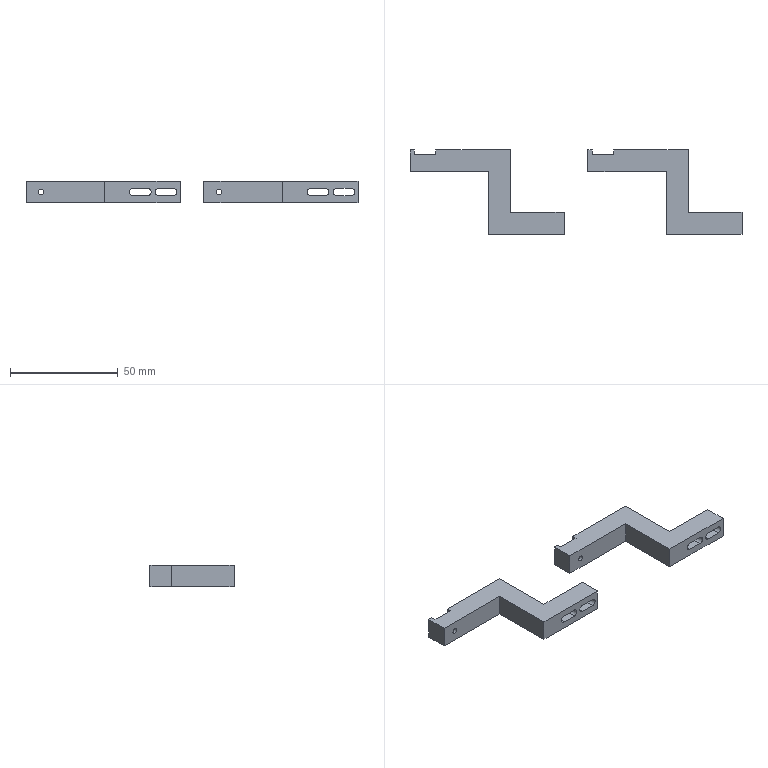Part | 2 solids | 46 faces | box 154 x 39 x 10 mm | volume 18361 mm3 | plane 36 | cylinder 10 | commonest cylinder face diameters 3.4 x8 2.5 x2
STEP:
#1=CARTESIAN_POINT('',(-3.2,10.,6.7));
#2=VERTEX_POINT('',#1);
#3=CARTESIAN_POINT('',(-3.2,0.,6.7));
#4=VERTEX_POINT('',#3);
#5=CARTESIAN_POINT('',(-3.2,10.,6.7));
#6=DIRECTION('',(0.,-1.,0.));
#7=VECTOR('',#6,1000.);
#8=LINE('',#5,#7);
#9=EDGE_CURVE('',#2,#4,#8,.T.);
#10=ORIENTED_EDGE('',*,*,#9,.T.);
#11=CARTESIAN_POINT('',(-9.8,0.,6.7));
#12=VERTEX_POINT('',#11);
#13=CARTESIAN_POINT('',(-9.8,0.,6.7));
#14=DIRECTION('',(1.,0.,0.));
#15=VECTOR('',#14,1000.);
#16=LINE('',#13,#15);
#17=EDGE_CURVE('',#12,#4,#16,.T.);
#18=ORIENTED_EDGE('',*,*,#17,.F.);
#19=CARTESIAN_POINT('',(-9.8,10.,6.7));
#20=VERTEX_POINT('',#19);
#21=CARTESIAN_POINT('',(-9.8,10.,6.7));
#22=DIRECTION('',(0.,1.,0.));
#23=VECTOR('',#22,1000.);
#24=LINE('',#21,#23);
#25=EDGE_CURVE('',#12,#20,#24,.T.);
#26=ORIENTED_EDGE('',*,*,#25,.T.);
#27=CARTESIAN_POINT('',(-9.8,10.,6.7));
#28=DIRECTION('',(1.,0.,0.));
#29=VECTOR('',#28,1000.);
#30=LINE('',#27,#29);
#31=EDGE_CURVE('',#20,#2,#30,.T.);
#32=ORIENTED_EDGE('',*,*,#31,.T.);
#33=EDGE_LOOP('',(#10,#18,#26,#32));
#34=FACE_BOUND('',#33,.T.);
#35=CARTESIAN_POINT('',(-9.8,10.,6.7));
#36=DIRECTION('',(0.,0.,1.));
#37=DIRECTION('',(1.,0.,0.));
#38=AXIS2_PLACEMENT_3D('',#35,#36,#37);
#39=PLANE('',#38);
#40=ADVANCED_FACE('',(#34),#39,.F.);
#41=CARTESIAN_POINT('',(-3.2,0.,3.3));
#42=VERTEX_POINT('',#41);
#43=CARTESIAN_POINT('',(-3.2,10.,3.3));
#44=VERTEX_POINT('',#43);
#45=CARTESIAN_POINT('',(-3.2,10.,3.3));
#46=DIRECTION('',(0.,1.,0.));
#47=VECTOR('',#46,1000.);
#48=LINE('',#45,#47);
#49=EDGE_CURVE('',#42,#44,#48,.T.);
#50=ORIENTED_EDGE('',*,*,#49,.T.);
#51=CARTESIAN_POINT('',(-9.8,10.,3.3));
#52=VERTEX_POINT('',#51);
#53=CARTESIAN_POINT('',(-9.8,10.,3.3));
#54=DIRECTION('',(1.,0.,0.));
#55=VECTOR('',#54,1000.);
#56=LINE('',#53,#55);
#57=EDGE_CURVE('',#52,#44,#56,.T.);
#58=ORIENTED_EDGE('',*,*,#57,.F.);
#59=CARTESIAN_POINT('',(-9.8,0.,3.3));
#60=VERTEX_POINT('',#59);
#61=CARTESIAN_POINT('',(-9.8,10.,3.3));
#62=DIRECTION('',(0.,-1.,0.));
#63=VECTOR('',#62,1000.);
#64=LINE('',#61,#63);
#65=EDGE_CURVE('',#52,#60,#64,.T.);
#66=ORIENTED_EDGE('',*,*,#65,.T.);
#67=CARTESIAN_POINT('',(-9.8,0.,3.3));
#68=DIRECTION('',(1.,0.,0.));
#69=VECTOR('',#68,1000.);
#70=LINE('',#67,#69);
#71=EDGE_CURVE('',#60,#42,#70,.T.);
#72=ORIENTED_EDGE('',*,*,#71,.T.);
#73=EDGE_LOOP('',(#50,#58,#66,#72));
#74=FACE_BOUND('',#73,.T.);
#75=CARTESIAN_POINT('',(-9.8,10.,3.3));
#76=DIRECTION('',(0.,0.,-1.));
#77=DIRECTION('',(-1.,0.,0.));
#78=AXIS2_PLACEMENT_3D('',#75,#76,#77);
#79=PLANE('',#78);
#80=ADVANCED_FACE('',(#74),#79,.F.);
#81=CARTESIAN_POINT('',(-9.8,10.,5.));
#82=DIRECTION('',(0.,1.,0.));
#83=DIRECTION('',(0.,0.,1.));
#84=AXIS2_PLACEMENT_3D('',#81,#82,#83);
#85=CIRCLE('',#84,1.7);
#86=EDGE_CURVE('',#52,#20,#85,.T.);
#87=ORIENTED_EDGE('',*,*,#86,.T.);
#88=ORIENTED_EDGE('',*,*,#25,.F.);
#89=CARTESIAN_POINT('',(-9.8,0.,5.));
#90=DIRECTION('',(0.,1.,0.));
#91=DIRECTION('',(0.,0.,1.));
#92=AXIS2_PLACEMENT_3D('',#89,#90,#91);
#93=CIRCLE('',#92,1.7);
#94=EDGE_CURVE('',#60,#12,#93,.T.);
#95=ORIENTED_EDGE('',*,*,#94,.F.);
#96=ORIENTED_EDGE('',*,*,#65,.F.);
#97=EDGE_LOOP('',(#87,#88,#95,#96));
#98=FACE_BOUND('',#97,.T.);
#99=CARTESIAN_POINT('',(-9.8,10.,5.));
#100=DIRECTION('',(0.,1.,0.));
#101=DIRECTION('',(0.,0.,1.));
#102=AXIS2_PLACEMENT_3D('',#99,#100,#101);
#103=CYLINDRICAL_SURFACE('',#102,1.7);
#104=ADVANCED_FACE('',(#98),#103,.F.);
#105=CARTESIAN_POINT('',(-3.2,0.,5.));
#106=DIRECTION('',(0.,1.,0.));
#107=DIRECTION('',(0.,0.,1.));
#108=AXIS2_PLACEMENT_3D('',#105,#106,#107);
#109=CIRCLE('',#108,1.7);
#110=EDGE_CURVE('',#4,#42,#109,.T.);
#111=ORIENTED_EDGE('',*,*,#110,.F.);
#112=ORIENTED_EDGE('',*,*,#9,.F.);
#113=CARTESIAN_POINT('',(-3.2,10.,5.));
#114=DIRECTION('',(0.,1.,0.));
#115=DIRECTION('',(0.,0.,1.));
#116=AXIS2_PLACEMENT_3D('',#113,#114,#115);
#117=CIRCLE('',#116,1.7);
#118=EDGE_CURVE('',#2,#44,#117,.T.);
#119=ORIENTED_EDGE('',*,*,#118,.T.);
#120=ORIENTED_EDGE('',*,*,#49,.F.);
#121=EDGE_LOOP('',(#111,#112,#119,#120));
#122=FACE_BOUND('',#121,.T.);
#123=CARTESIAN_POINT('',(-3.2,10.,5.));
#124=DIRECTION('',(0.,1.,0.));
#125=DIRECTION('',(0.,0.,1.));
#126=AXIS2_PLACEMENT_3D('',#123,#124,#125);
#127=CYLINDRICAL_SURFACE('',#126,1.7);
#128=ADVANCED_FACE('',(#122),#127,.F.);
#129=CARTESIAN_POINT('',(-15.2,10.,6.7));
#130=VERTEX_POINT('',#129);
#131=CARTESIAN_POINT('',(-15.2,0.,6.7));
#132=VERTEX_POINT('',#131);
#133=CARTESIAN_POINT('',(-15.2,10.,6.7));
#134=DIRECTION('',(0.,-1.,0.));
#135=VECTOR('',#134,1000.);
#136=LINE('',#133,#135);
#137=EDGE_CURVE('',#130,#132,#136,.T.);
#138=ORIENTED_EDGE('',*,*,#137,.T.);
#139=CARTESIAN_POINT('',(-21.8,0.,6.7));
#140=VERTEX_POINT('',#139);
#141=CARTESIAN_POINT('',(-35.,0.,6.7));
#142=DIRECTION('',(1.,0.,0.));
#143=VECTOR('',#142,1000.);
#144=LINE('',#141,#143);
#145=EDGE_CURVE('',#140,#132,#144,.T.);
#146=ORIENTED_EDGE('',*,*,#145,.F.);
#147=CARTESIAN_POINT('',(-21.8,10.,6.7));
#148=VERTEX_POINT('',#147);
#149=CARTESIAN_POINT('',(-21.8,10.,6.7));
#150=DIRECTION('',(0.,1.,0.));
#151=VECTOR('',#150,1000.);
#152=LINE('',#149,#151);
#153=EDGE_CURVE('',#140,#148,#152,.T.);
#154=ORIENTED_EDGE('',*,*,#153,.T.);
#155=CARTESIAN_POINT('',(-9.8,10.,6.7));
#156=DIRECTION('',(1.,0.,0.));
#157=VECTOR('',#156,1000.);
#158=LINE('',#155,#157);
#159=EDGE_CURVE('',#148,#130,#158,.T.);
#160=ORIENTED_EDGE('',*,*,#159,.T.);
#161=EDGE_LOOP('',(#138,#146,#154,#160));
#162=FACE_BOUND('',#161,.T.);
#163=CARTESIAN_POINT('',(-9.8,10.,6.7));
#164=DIRECTION('',(0.,0.,1.));
#165=DIRECTION('',(1.,0.,0.));
#166=AXIS2_PLACEMENT_3D('',#163,#164,#165);
#167=PLANE('',#166);
#168=ADVANCED_FACE('',(#162),#167,.F.);
#169=CARTESIAN_POINT('',(-15.2,0.,3.3));
#170=VERTEX_POINT('',#169);
#171=CARTESIAN_POINT('',(-15.2,10.,3.3));
#172=VERTEX_POINT('',#171);
#173=CARTESIAN_POINT('',(-15.2,10.,3.3));
#174=DIRECTION('',(0.,1.,0.));
#175=VECTOR('',#174,1000.);
#176=LINE('',#173,#175);
#177=EDGE_CURVE('',#170,#172,#176,.T.);
#178=ORIENTED_EDGE('',*,*,#177,.T.);
#179=CARTESIAN_POINT('',(-21.8,10.,3.3));
#180=VERTEX_POINT('',#179);
#181=CARTESIAN_POINT('',(0.,10.,3.3));
#182=DIRECTION('',(1.,0.,0.));
#183=VECTOR('',#182,1000.);
#184=LINE('',#181,#183);
#185=EDGE_CURVE('',#180,#172,#184,.T.);
#186=ORIENTED_EDGE('',*,*,#185,.F.);
#187=CARTESIAN_POINT('',(-21.8,0.,3.3));
#188=VERTEX_POINT('',#187);
#189=CARTESIAN_POINT('',(-21.8,10.,3.3));
#190=DIRECTION('',(0.,-1.,0.));
#191=VECTOR('',#190,1000.);
#192=LINE('',#189,#191);
#193=EDGE_CURVE('',#180,#188,#192,.T.);
#194=ORIENTED_EDGE('',*,*,#193,.T.);
#195=CARTESIAN_POINT('',(-9.8,0.,3.3));
#196=DIRECTION('',(1.,0.,0.));
#197=VECTOR('',#196,1000.);
#198=LINE('',#195,#197);
#199=EDGE_CURVE('',#188,#170,#198,.T.);
#200=ORIENTED_EDGE('',*,*,#199,.T.);
#201=EDGE_LOOP('',(#178,#186,#194,#200));
#202=FACE_BOUND('',#201,.T.);
#203=CARTESIAN_POINT('',(-9.8,10.,3.3));
#204=DIRECTION('',(0.,0.,-1.));
#205=DIRECTION('',(-1.,0.,0.));
#206=AXIS2_PLACEMENT_3D('',#203,#204,#205);
#207=PLANE('',#206);
#208=ADVANCED_FACE('',(#202),#207,.F.);
#209=CARTESIAN_POINT('',(-21.8,10.,5.));
#210=DIRECTION('',(0.,1.,0.));
#211=DIRECTION('',(0.,0.,1.));
#212=AXIS2_PLACEMENT_3D('',#209,#210,#211);
#213=CIRCLE('',#212,1.7);
#214=EDGE_CURVE('',#180,#148,#213,.T.);
#215=ORIENTED_EDGE('',*,*,#214,.T.);
#216=ORIENTED_EDGE('',*,*,#153,.F.);
#217=CARTESIAN_POINT('',(-21.8,0.,5.));
#218=DIRECTION('',(0.,1.,0.));
#219=DIRECTION('',(0.,0.,1.));
#220=AXIS2_PLACEMENT_3D('',#217,#218,#219);
#221=CIRCLE('',#220,1.7);
#222=EDGE_CURVE('',#188,#140,#221,.T.);
#223=ORIENTED_EDGE('',*,*,#222,.F.);
#224=ORIENTED_EDGE('',*,*,#193,.F.);
#225=EDGE_LOOP('',(#215,#216,#223,#224));
#226=FACE_BOUND('',#225,.T.);
#227=CARTESIAN_POINT('',(-21.8,10.,5.));
#228=DIRECTION('',(0.,1.,0.));
#229=DIRECTION('',(0.,0.,1.));
#230=AXIS2_PLACEMENT_3D('',#227,#228,#229);
#231=CYLINDRICAL_SURFACE('',#230,1.7);
#232=ADVANCED_FACE('',(#226),#231,.F.);
#233=CARTESIAN_POINT('',(-15.2,0.,5.));
#234=DIRECTION('',(0.,1.,0.));
#235=DIRECTION('',(0.,0.,1.));
#236=AXIS2_PLACEMENT_3D('',#233,#234,#235);
#237=CIRCLE('',#236,1.7);
#238=EDGE_CURVE('',#132,#170,#237,.T.);
#239=ORIENTED_EDGE('',*,*,#238,.F.);
#240=ORIENTED_EDGE('',*,*,#137,.F.);
#241=CARTESIAN_POINT('',(-15.2,10.,5.));
#242=DIRECTION('',(0.,1.,0.));
#243=DIRECTION('',(0.,0.,1.));
#244=AXIS2_PLACEMENT_3D('',#241,#242,#243);
#245=CIRCLE('',#244,1.7);
#246=EDGE_CURVE('',#130,#172,#245,.T.);
#247=ORIENTED_EDGE('',*,*,#246,.T.);
#248=ORIENTED_EDGE('',*,*,#177,.F.);
#249=EDGE_LOOP('',(#239,#240,#247,#248));
#250=FACE_BOUND('',#249,.T.);
#251=CARTESIAN_POINT('',(-15.2,10.,5.));
#252=DIRECTION('',(0.,1.,0.));
#253=DIRECTION('',(0.,0.,1.));
#254=AXIS2_PLACEMENT_3D('',#251,#252,#253);
#255=CYLINDRICAL_SURFACE('',#254,1.7);
#256=ADVANCED_FACE('',(#250),#255,.F.);
#257=CARTESIAN_POINT('',(-25.,10.,0.));
#258=VERTEX_POINT('',#257);
#259=CARTESIAN_POINT('',(-25.,39.,0.));
#260=VERTEX_POINT('',#259);
#261=CARTESIAN_POINT('',(-25.,39.,0.));
#262=DIRECTION('',(0.,1.,0.));
#263=VECTOR('',#262,1000.);
#264=LINE('',#261,#263);
#265=EDGE_CURVE('',#258,#260,#264,.T.);
#266=ORIENTED_EDGE('',*,*,#265,.T.);
#267=CARTESIAN_POINT('',(-25.,39.,10.));
#268=VERTEX_POINT('',#267);
#269=CARTESIAN_POINT('',(-25.,39.,10.));
#270=DIRECTION('',(0.,0.,-1.));
#271=VECTOR('',#270,1000.);
#272=LINE('',#269,#271);
#273=EDGE_CURVE('',#268,#260,#272,.T.);
#274=ORIENTED_EDGE('',*,*,#273,.F.);
#275=CARTESIAN_POINT('',(-25.,10.,10.));
#276=VERTEX_POINT('',#275);
#277=CARTESIAN_POINT('',(-25.,39.,10.));
#278=DIRECTION('',(0.,1.,0.));
#279=VECTOR('',#278,1000.);
#280=LINE('',#277,#279);
#281=EDGE_CURVE('',#276,#268,#280,.T.);
#282=ORIENTED_EDGE('',*,*,#281,.F.);
#283=CARTESIAN_POINT('',(-25.,10.,10.));
#284=DIRECTION('',(0.,0.,-1.));
#285=VECTOR('',#284,1000.);
#286=LINE('',#283,#285);
#287=EDGE_CURVE('',#276,#258,#286,.T.);
#288=ORIENTED_EDGE('',*,*,#287,.T.);
#289=EDGE_LOOP('',(#266,#274,#282,#288));
#290=FACE_BOUND('',#289,.T.);
#291=CARTESIAN_POINT('',(-25.,39.,10.));
#292=DIRECTION('',(-1.,0.,0.));
#293=DIRECTION('',(0.,-1.,0.));
#294=AXIS2_PLACEMENT_3D('',#291,#292,#293);
#295=PLANE('',#294);
#296=ADVANCED_FACE('',(#290),#295,.F.);
#297=CARTESIAN_POINT('',(-69.5,37.,0.));
#298=VERTEX_POINT('',#297);
#299=CARTESIAN_POINT('',(-69.5,37.,10.));
#300=VERTEX_POINT('',#299);
#301=CARTESIAN_POINT('',(-69.5,37.,0.));
#302=DIRECTION('',(0.,0.,1.));
#303=VECTOR('',#302,1000.);
#304=LINE('',#301,#303);
#305=EDGE_CURVE('',#298,#300,#304,.T.);
#306=ORIENTED_EDGE('',*,*,#305,.T.);
#307=CARTESIAN_POINT('',(-59.5,37.,10.));
#308=VERTEX_POINT('',#307);
#309=CARTESIAN_POINT('',(-69.5,37.,10.));
#310=DIRECTION('',(1.,0.,0.));
#311=VECTOR('',#310,1000.);
#312=LINE('',#309,#311);
#313=EDGE_CURVE('',#300,#308,#312,.T.);
#314=ORIENTED_EDGE('',*,*,#313,.T.);
#315=CARTESIAN_POINT('',(-59.5,37.,0.));
#316=VERTEX_POINT('',#315);
#317=CARTESIAN_POINT('',(-59.5,37.,0.));
#318=DIRECTION('',(0.,0.,-1.));
#319=VECTOR('',#318,1000.);
#320=LINE('',#317,#319);
#321=EDGE_CURVE('',#308,#316,#320,.T.);
#322=ORIENTED_EDGE('',*,*,#321,.T.);
#323=CARTESIAN_POINT('',(-69.5,37.,0.));
#324=DIRECTION('',(-1.,0.,0.));
#325=VECTOR('',#324,1000.);
#326=LINE('',#323,#325);
#327=EDGE_CURVE('',#316,#298,#326,.T.);
#328=ORIENTED_EDGE('',*,*,#327,.T.);
#329=EDGE_LOOP('',(#306,#314,#322,#328));
#330=FACE_BOUND('',#329,.T.);
#331=CARTESIAN_POINT('',(-64.5,37.,6.25));
#332=VERTEX_POINT('',#331);
#333=CARTESIAN_POINT('',(-64.5,37.,5.));
#334=DIRECTION('',(0.,1.,0.));
#335=DIRECTION('',(0.,0.,1.));
#336=AXIS2_PLACEMENT_3D('',#333,#334,#335);
#337=CIRCLE('',#336,1.25);
#338=EDGE_CURVE('',#332,#332,#337,.T.);
#339=ORIENTED_EDGE('',*,*,#338,.F.);
#340=EDGE_LOOP('',(#339));
#341=FACE_BOUND('',#340,.T.);
#342=CARTESIAN_POINT('',(0.,37.,0.));
#343=DIRECTION('',(0.,1.,0.));
#344=DIRECTION('',(-1.,0.,0.));
#345=AXIS2_PLACEMENT_3D('',#342,#343,#344);
#346=PLANE('',#345);
#347=ADVANCED_FACE('',(#330,#341),#346,.T.);
#348=CARTESIAN_POINT('',(-59.5,39.,10.));
#349=VERTEX_POINT('',#348);
#350=CARTESIAN_POINT('',(-59.5,39.,0.));
#351=VERTEX_POINT('',#350);
#352=CARTESIAN_POINT('',(-59.5,39.,0.));
#353=DIRECTION('',(0.,0.,-1.));
#354=VECTOR('',#353,1000.);
#355=LINE('',#352,#354);
#356=EDGE_CURVE('',#349,#351,#355,.T.);
#357=ORIENTED_EDGE('',*,*,#356,.T.);
#358=CARTESIAN_POINT('',(-59.5,37.,0.));
#359=DIRECTION('',(0.,1.,0.));
#360=VECTOR('',#359,1000.);
#361=LINE('',#358,#360);
#362=EDGE_CURVE('',#316,#351,#361,.T.);
#363=ORIENTED_EDGE('',*,*,#362,.F.);
#364=ORIENTED_EDGE('',*,*,#321,.F.);
#365=CARTESIAN_POINT('',(-59.5,37.,10.));
#366=DIRECTION('',(0.,1.,0.));
#367=VECTOR('',#366,1000.);
#368=LINE('',#365,#367);
#369=EDGE_CURVE('',#308,#349,#368,.T.);
#370=ORIENTED_EDGE('',*,*,#369,.T.);
#371=EDGE_LOOP('',(#357,#363,#364,#370));
#372=FACE_BOUND('',#371,.T.);
#373=CARTESIAN_POINT('',(-59.5,37.,0.));
#374=DIRECTION('',(1.,0.,0.));
#375=DIRECTION('',(0.,1.,0.));
#376=AXIS2_PLACEMENT_3D('',#373,#374,#375);
#377=PLANE('',#376);
#378=ADVANCED_FACE('',(#372),#377,.F.);
#379=CARTESIAN_POINT('',(-69.5,39.,0.));
#380=VERTEX_POINT('',#379);
#381=CARTESIAN_POINT('',(-69.5,39.,10.));
#382=VERTEX_POINT('',#381);
#383=CARTESIAN_POINT('',(-69.5,39.,0.));
#384=DIRECTION('',(0.,0.,1.));
#385=VECTOR('',#384,1000.);
#386=LINE('',#383,#385);
#387=EDGE_CURVE('',#380,#382,#386,.T.);
#388=ORIENTED_EDGE('',*,*,#387,.T.);
#389=CARTESIAN_POINT('',(-69.5,37.,10.));
#390=DIRECTION('',(0.,1.,0.));
#391=VECTOR('',#390,1000.);
#392=LINE('',#389,#391);
#393=EDGE_CURVE('',#300,#382,#392,.T.);
#394=ORIENTED_EDGE('',*,*,#393,.F.);
#395=ORIENTED_EDGE('',*,*,#305,.F.);
#396=CARTESIAN_POINT('',(-69.5,37.,0.));
#397=DIRECTION('',(0.,1.,0.));
#398=VECTOR('',#397,1000.);
#399=LINE('',#396,#398);
#400=EDGE_CURVE('',#298,#380,#399,.T.);
#401=ORIENTED_EDGE('',*,*,#400,.T.);
#402=EDGE_LOOP('',(#388,#394,#395,#401));
#403=FACE_BOUND('',#402,.T.);
#404=CARTESIAN_POINT('',(-69.5,37.,0.));
#405=DIRECTION('',(-1.,0.,0.));
#406=DIRECTION('',(0.,-1.,0.));
#407=AXIS2_PLACEMENT_3D('',#404,#405,#406);
#408=PLANE('',#407);
#409=ADVANCED_FACE('',(#403),#408,.F.);
#410=CARTESIAN_POINT('',(0.,39.,0.));
#411=DIRECTION('',(-1.,0.,0.));
#412=VECTOR('',#411,1000.);
#413=LINE('',#410,#412);
#414=EDGE_CURVE('',#260,#351,#413,.T.);
#415=ORIENTED_EDGE('',*,*,#414,.F.);
#416=ORIENTED_EDGE('',*,*,#265,.F.);
#417=CARTESIAN_POINT('',(0.,10.,0.));
#418=VERTEX_POINT('',#417);
#419=CARTESIAN_POINT('',(0.,10.,0.));
#420=DIRECTION('',(-1.,0.,0.));
#421=VECTOR('',#420,1000.);
#422=LINE('',#419,#421);
#423=EDGE_CURVE('',#418,#258,#422,.T.);
#424=ORIENTED_EDGE('',*,*,#423,.F.);
#425=CARTESIAN_POINT('',(0.,0.,0.));
#426=VERTEX_POINT('',#425);
#427=CARTESIAN_POINT('',(0.,0.,0.));
#428=DIRECTION('',(0.,1.,0.));
#429=VECTOR('',#428,1000.);
#430=LINE('',#427,#429);
#431=EDGE_CURVE('',#426,#418,#430,.T.);
#432=ORIENTED_EDGE('',*,*,#431,.F.);
#433=CARTESIAN_POINT('',(-35.,0.,0.));
#434=VERTEX_POINT('',#433);
#435=CARTESIAN_POINT('',(-35.,0.,0.));
#436=DIRECTION('',(1.,0.,0.));
#437=VECTOR('',#436,1000.);
#438=LINE('',#435,#437);
#439=EDGE_CURVE('',#434,#426,#438,.T.);
#440=ORIENTED_EDGE('',*,*,#439,.F.);
#441=CARTESIAN_POINT('',(-35.,29.,0.));
#442=VERTEX_POINT('',#441);
#443=CARTESIAN_POINT('',(-35.,29.,0.));
#444=DIRECTION('',(0.,-1.,0.));
#445=VECTOR('',#444,1000.);
#446=LINE('',#443,#445);
#447=EDGE_CURVE('',#442,#434,#446,.T.);
#448=ORIENTED_EDGE('',*,*,#447,.F.);
#449=CARTESIAN_POINT('',(-71.5,29.,0.));
#450=VERTEX_POINT('',#449);
#451=CARTESIAN_POINT('',(-71.5,29.,0.));
#452=DIRECTION('',(1.,0.,0.));
#453=VECTOR('',#452,1000.);
#454=LINE('',#451,#453);
#455=EDGE_CURVE('',#450,#442,#454,.T.);
#456=ORIENTED_EDGE('',*,*,#455,.F.);
#457=CARTESIAN_POINT('',(-71.5,39.,0.));
#458=VERTEX_POINT('',#457);
#459=CARTESIAN_POINT('',(-71.5,39.,0.));
#460=DIRECTION('',(0.,-1.,0.));
#461=VECTOR('',#460,1000.);
#462=LINE('',#459,#461);
#463=EDGE_CURVE('',#458,#450,#462,.T.);
#464=ORIENTED_EDGE('',*,*,#463,.F.);
#465=CARTESIAN_POINT('',(0.,39.,0.));
#466=DIRECTION('',(-1.,0.,0.));
#467=VECTOR('',#466,1000.);
#468=LINE('',#465,#467);
#469=EDGE_CURVE('',#380,#458,#468,.T.);
#470=ORIENTED_EDGE('',*,*,#469,.F.);
#471=ORIENTED_EDGE('',*,*,#400,.F.);
#472=ORIENTED_EDGE('',*,*,#327,.F.);
#473=ORIENTED_EDGE('',*,*,#362,.T.);
#474=EDGE_LOOP('',(#415,#416,#424,#432,#440,#448,#456,#464,#470,#471,#472,#473));
#475=FACE_BOUND('',#474,.T.);
#476=CARTESIAN_POINT('',(0.,0.,0.));
#477=DIRECTION('',(0.,0.,1.));
#478=DIRECTION('',(1.,0.,0.));
#479=AXIS2_PLACEMENT_3D('',#476,#477,#478);
#480=PLANE('',#479);
#481=ADVANCED_FACE('',(#475),#480,.F.);
#482=ORIENTED_EDGE('',*,*,#281,.T.);
#483=CARTESIAN_POINT('',(0.,39.,10.));
#484=DIRECTION('',(-1.,0.,0.));
#485=VECTOR('',#484,1000.);
#486=LINE('',#483,#485);
#487=EDGE_CURVE('',#268,#349,#486,.T.);
#488=ORIENTED_EDGE('',*,*,#487,.T.);
#489=ORIENTED_EDGE('',*,*,#369,.F.);
#490=ORIENTED_EDGE('',*,*,#313,.F.);
#491=ORIENTED_EDGE('',*,*,#393,.T.);
#492=CARTESIAN_POINT('',(-71.5,39.,10.));
#493=VERTEX_POINT('',#492);
#494=CARTESIAN_POINT('',(0.,39.,10.));
#495=DIRECTION('',(-1.,0.,0.));
#496=VECTOR('',#495,1000.);
#497=LINE('',#494,#496);
#498=EDGE_CURVE('',#382,#493,#497,.T.);
#499=ORIENTED_EDGE('',*,*,#498,.T.);
#500=CARTESIAN_POINT('',(-71.5,29.,10.));
#501=VERTEX_POINT('',#500);
#502=CARTESIAN_POINT('',(-71.5,39.,10.));
#503=DIRECTION('',(0.,-1.,0.));
#504=VECTOR('',#503,1000.);
#505=LINE('',#502,#504);
#506=EDGE_CURVE('',#493,#501,#505,.T.);
#507=ORIENTED_EDGE('',*,*,#506,.T.);
#508=CARTESIAN_POINT('',(-35.,29.,10.));
#509=VERTEX_POINT('',#508);
#510=CARTESIAN_POINT('',(-71.5,29.,10.));
#511=DIRECTION('',(1.,0.,0.));
#512=VECTOR('',#511,1000.);
#513=LINE('',#510,#512);
#514=EDGE_CURVE('',#501,#509,#513,.T.);
#515=ORIENTED_EDGE('',*,*,#514,.T.);
#516=CARTESIAN_POINT('',(-35.,0.,10.));
#517=VERTEX_POINT('',#516);
#518=CARTESIAN_POINT('',(-35.,29.,10.));
#519=DIRECTION('',(0.,-1.,0.));
#520=VECTOR('',#519,1000.);
#521=LINE('',#518,#520);
#522=EDGE_CURVE('',#509,#517,#521,.T.);
#523=ORIENTED_EDGE('',*,*,#522,.T.);
#524=CARTESIAN_POINT('',(0.,0.,10.));
#525=VERTEX_POINT('',#524);
#526=CARTESIAN_POINT('',(-35.,0.,10.));
#527=DIRECTION('',(1.,0.,0.));
#528=VECTOR('',#527,1000.);
#529=LINE('',#526,#528);
#530=EDGE_CURVE('',#517,#525,#529,.T.);
#531=ORIENTED_EDGE('',*,*,#530,.T.);
#532=CARTESIAN_POINT('',(0.,10.,10.));
#533=VERTEX_POINT('',#532);
#534=CARTESIAN_POINT('',(0.,0.,10.));
#535=DIRECTION('',(0.,1.,0.));
#536=VECTOR('',#535,1000.);
#537=LINE('',#534,#536);
#538=EDGE_CURVE('',#525,#533,#537,.T.);
#539=ORIENTED_EDGE('',*,*,#538,.T.);
#540=CARTESIAN_POINT('',(0.,10.,10.));
#541=DIRECTION('',(-1.,0.,0.));
#542=VECTOR('',#541,1000.);
#543=LINE('',#540,#542);
#544=EDGE_CURVE('',#533,#276,#543,.T.);
#545=ORIENTED_EDGE('',*,*,#544,.T.);
#546=EDGE_LOOP('',(#482,#488,#489,#490,#491,#499,#507,#515,#523,#531,#539,#545));
#547=FACE_BOUND('',#546,.T.);
#548=CARTESIAN_POINT('',(0.,0.,10.));
#549=DIRECTION('',(0.,0.,1.));
#550=DIRECTION('',(1.,0.,0.));
#551=AXIS2_PLACEMENT_3D('',#548,#549,#550);
#552=PLANE('',#551);
#553=ADVANCED_FACE('',(#547),#552,.T.);
#554=ORIENTED_EDGE('',*,*,#447,.T.);
#555=CARTESIAN_POINT('',(-35.,0.,10.));
#556=DIRECTION('',(0.,0.,-1.));
#557=VECTOR('',#556,1000.);
#558=LINE('',#555,#557);
#559=EDGE_CURVE('',#517,#434,#558,.T.);
#560=ORIENTED_EDGE('',*,*,#559,.F.);
#561=ORIENTED_EDGE('',*,*,#522,.F.);
#562=CARTESIAN_POINT('',(-35.,29.,10.));
#563=DIRECTION('',(0.,0.,-1.));
#564=VECTOR('',#563,1000.);
#565=LINE('',#562,#564);
#566=EDGE_CURVE('',#509,#442,#565,.T.);
#567=ORIENTED_EDGE('',*,*,#566,.T.);
#568=EDGE_LOOP('',(#554,#560,#561,#567));
#569=FACE_BOUND('',#568,.T.);
#570=CARTESIAN_POINT('',(-35.,29.,10.));
#571=DIRECTION('',(1.,0.,0.));
#572=DIRECTION('',(0.,1.,0.));
#573=AXIS2_PLACEMENT_3D('',#570,#571,#572);
#574=PLANE('',#573);
#575=ADVANCED_FACE('',(#569),#574,.F.);
#576=ORIENTED_EDGE('',*,*,#455,.T.);
#577=ORIENTED_EDGE('',*,*,#566,.F.);
#578=ORIENTED_EDGE('',*,*,#514,.F.);
#579=CARTESIAN_POINT('',(-71.5,29.,10.));
#580=DIRECTION('',(0.,0.,-1.));
#581=VECTOR('',#580,1000.);
#582=LINE('',#579,#581);
#583=EDGE_CURVE('',#501,#450,#582,.T.);
#584=ORIENTED_EDGE('',*,*,#583,.T.);
#585=EDGE_LOOP('',(#576,#577,#578,#584));
#586=FACE_BOUND('',#585,.T.);
#587=CARTESIAN_POINT('',(-64.5,29.,6.25));
#588=VERTEX_POINT('',#587);
#589=CARTESIAN_POINT('',(-64.5,29.,5.));
#590=DIRECTION('',(0.,1.,0.));
#591=DIRECTION('',(0.,0.,1.));
#592=AXIS2_PLACEMENT_3D('',#589,#590,#591);
#593=CIRCLE('',#592,1.25);
#594=EDGE_CURVE('',#588,#588,#593,.T.);
#595=ORIENTED_EDGE('',*,*,#594,.T.);
#596=EDGE_LOOP('',(#595));
#597=FACE_BOUND('',#596,.T.);
#598=CARTESIAN_POINT('',(-71.5,29.,10.));
#599=DIRECTION('',(0.,1.,0.));
#600=DIRECTION('',(0.,0.,1.));
#601=AXIS2_PLACEMENT_3D('',#598,#599,#600);
#602=PLANE('',#601);
#603=ADVANCED_FACE('',(#586,#597),#602,.F.);
#604=ORIENTED_EDGE('',*,*,#463,.T.);
#605=ORIENTED_EDGE('',*,*,#583,.F.);
#606=ORIENTED_EDGE('',*,*,#506,.F.);
#607=CARTESIAN_POINT('',(-71.5,39.,10.));
#608=DIRECTION('',(0.,0.,-1.));
#609=VECTOR('',#608,1000.);
#610=LINE('',#607,#609);
#611=EDGE_CURVE('',#493,#458,#610,.T.);
#612=ORIENTED_EDGE('',*,*,#611,.T.);
#613=EDGE_LOOP('',(#604,#605,#606,#612));
#614=FACE_BOUND('',#613,.T.);
#615=CARTESIAN_POINT('',(-71.5,39.,10.));
#616=DIRECTION('',(1.,0.,0.));
#617=DIRECTION('',(0.,1.,0.));
#618=AXIS2_PLACEMENT_3D('',#615,#616,#617);
#619=PLANE('',#618);
#620=ADVANCED_FACE('',(#614),#619,.F.);
#621=ORIENTED_EDGE('',*,*,#487,.F.);
#622=ORIENTED_EDGE('',*,*,#273,.T.);
#623=ORIENTED_EDGE('',*,*,#414,.T.);
#624=ORIENTED_EDGE('',*,*,#356,.F.);
#625=EDGE_LOOP('',(#621,#622,#623,#624));
#626=FACE_BOUND('',#625,.T.);
#627=CARTESIAN_POINT('',(0.,39.,10.));
#628=DIRECTION('',(0.,-1.,0.));
#629=DIRECTION('',(0.,0.,-1.));
#630=AXIS2_PLACEMENT_3D('',#627,#628,#629);
#631=PLANE('',#630);
#632=ADVANCED_FACE('',(#626),#631,.F.);
#633=ORIENTED_EDGE('',*,*,#431,.T.);
#634=CARTESIAN_POINT('',(0.,10.,10.));
#635=DIRECTION('',(0.,0.,-1.));
#636=VECTOR('',#635,1000.);
#637=LINE('',#634,#636);
#638=EDGE_CURVE('',#533,#418,#637,.T.);
#639=ORIENTED_EDGE('',*,*,#638,.F.);
#640=ORIENTED_EDGE('',*,*,#538,.F.);
#641=CARTESIAN_POINT('',(0.,0.,10.));
#642=DIRECTION('',(0.,0.,-1.));
#643=VECTOR('',#642,1000.);
#644=LINE('',#641,#643);
#645=EDGE_CURVE('',#525,#426,#644,.T.);
#646=ORIENTED_EDGE('',*,*,#645,.T.);
#647=EDGE_LOOP('',(#633,#639,#640,#646));
#648=FACE_BOUND('',#647,.T.);
#649=CARTESIAN_POINT('',(0.,0.,10.));
#650=DIRECTION('',(-1.,0.,0.));
#651=DIRECTION('',(0.,0.,1.));
#652=AXIS2_PLACEMENT_3D('',#649,#650,#651);
#653=PLANE('',#652);
#654=ADVANCED_FACE('',(#648),#653,.F.);
#655=ORIENTED_EDGE('',*,*,#439,.T.);
#656=ORIENTED_EDGE('',*,*,#645,.F.);
#657=ORIENTED_EDGE('',*,*,#530,.F.);
#658=ORIENTED_EDGE('',*,*,#559,.T.);
#659=EDGE_LOOP('',(#655,#656,#657,#658));
#660=FACE_BOUND('',#659,.T.);
#661=ORIENTED_EDGE('',*,*,#238,.T.);
#662=ORIENTED_EDGE('',*,*,#199,.F.);
#663=ORIENTED_EDGE('',*,*,#222,.T.);
#664=ORIENTED_EDGE('',*,*,#145,.T.);
#665=EDGE_LOOP('',(#661,#662,#663,#664));
#666=FACE_BOUND('',#665,.T.);
#667=ORIENTED_EDGE('',*,*,#17,.T.);
#668=ORIENTED_EDGE('',*,*,#110,.T.);
#669=ORIENTED_EDGE('',*,*,#71,.F.);
#670=ORIENTED_EDGE('',*,*,#94,.T.);
#671=EDGE_LOOP('',(#667,#668,#669,#670));
#672=FACE_BOUND('',#671,.T.);
#673=CARTESIAN_POINT('',(-35.,0.,10.));
#674=DIRECTION('',(0.,1.,0.));
#675=DIRECTION('',(0.,0.,1.));
#676=AXIS2_PLACEMENT_3D('',#673,#674,#675);
#677=PLANE('',#676);
#678=ADVANCED_FACE('',(#660,#666,#672),#677,.F.);
#679=ORIENTED_EDGE('',*,*,#498,.F.);
#680=ORIENTED_EDGE('',*,*,#387,.F.);
#681=ORIENTED_EDGE('',*,*,#469,.T.);
#682=ORIENTED_EDGE('',*,*,#611,.F.);
#683=EDGE_LOOP('',(#679,#680,#681,#682));
#684=FACE_BOUND('',#683,.T.);
#685=CARTESIAN_POINT('',(0.,39.,10.));
#686=DIRECTION('',(0.,-1.,0.));
#687=DIRECTION('',(0.,0.,-1.));
#688=AXIS2_PLACEMENT_3D('',#685,#686,#687);
#689=PLANE('',#688);
#690=ADVANCED_FACE('',(#684),#689,.F.);
#691=ORIENTED_EDGE('',*,*,#159,.F.);
#692=ORIENTED_EDGE('',*,*,#214,.F.);
#693=ORIENTED_EDGE('',*,*,#185,.T.);
#694=ORIENTED_EDGE('',*,*,#246,.F.);
#695=EDGE_LOOP('',(#691,#692,#693,#694));
#696=FACE_BOUND('',#695,.T.);
#697=ORIENTED_EDGE('',*,*,#423,.T.);
#698=ORIENTED_EDGE('',*,*,#287,.F.);
#699=ORIENTED_EDGE('',*,*,#544,.F.);
#700=ORIENTED_EDGE('',*,*,#638,.T.);
#701=EDGE_LOOP('',(#697,#698,#699,#700));
#702=FACE_BOUND('',#701,.T.);
#703=ORIENTED_EDGE('',*,*,#57,.T.);
#704=ORIENTED_EDGE('',*,*,#118,.F.);
#705=ORIENTED_EDGE('',*,*,#31,.F.);
#706=ORIENTED_EDGE('',*,*,#86,.F.);
#707=EDGE_LOOP('',(#703,#704,#705,#706));
#708=FACE_BOUND('',#707,.T.);
#709=CARTESIAN_POINT('',(0.,10.,10.));
#710=DIRECTION('',(0.,-1.,0.));
#711=DIRECTION('',(0.,0.,-1.));
#712=AXIS2_PLACEMENT_3D('',#709,#710,#711);
#713=PLANE('',#712);
#714=ADVANCED_FACE('',(#696,#702,#708),#713,.F.);
#715=ORIENTED_EDGE('',*,*,#594,.F.);
#716=EDGE_LOOP('',(#715));
#717=FACE_BOUND('',#716,.T.);
#718=ORIENTED_EDGE('',*,*,#338,.T.);
#719=EDGE_LOOP('',(#718));
#720=FACE_BOUND('',#719,.T.);
#721=CARTESIAN_POINT('',(-64.5,37.,5.));
#722=DIRECTION('',(0.,1.,0.));
#723=DIRECTION('',(0.,0.,1.));
#724=AXIS2_PLACEMENT_3D('',#721,#722,#723);
#725=CYLINDRICAL_SURFACE('',#724,1.25);
#726=ADVANCED_FACE('',(#717,#720),#725,.F.);
#727=CLOSED_SHELL('',(#40,#80,#104,#128,#168,#208,#232,#256,#296,#347,#378,#409,#481,#553,#575,#603,#620,#632,#654,#678,#690,#714,#726));
#728=MANIFOLD_SOLID_BREP('',#727);
#729=CARTESIAN_POINT('',(-85.7,10.,6.7));
#730=VERTEX_POINT('',#729);
#731=CARTESIAN_POINT('',(-85.7,0.,6.7));
#732=VERTEX_POINT('',#731);
#733=CARTESIAN_POINT('',(-85.7,10.,6.7));
#734=DIRECTION('',(0.,-1.,0.));
#735=VECTOR('',#734,1000.);
#736=LINE('',#733,#735);
#737=EDGE_CURVE('',#730,#732,#736,.T.);
#738=ORIENTED_EDGE('',*,*,#737,.T.);
#739=CARTESIAN_POINT('',(-92.3,0.,6.7));
#740=VERTEX_POINT('',#739);
#741=CARTESIAN_POINT('',(-92.3,0.,6.7));
#742=DIRECTION('',(1.,0.,0.));
#743=VECTOR('',#742,1000.);
#744=LINE('',#741,#743);
#745=EDGE_CURVE('',#740,#732,#744,.T.);
#746=ORIENTED_EDGE('',*,*,#745,.F.);
#747=CARTESIAN_POINT('',(-92.3,10.,6.7));
#748=VERTEX_POINT('',#747);
#749=CARTESIAN_POINT('',(-92.3,10.,6.7));
#750=DIRECTION('',(0.,1.,0.));
#751=VECTOR('',#750,1000.);
#752=LINE('',#749,#751);
#753=EDGE_CURVE('',#740,#748,#752,.T.);
#754=ORIENTED_EDGE('',*,*,#753,.T.);
#755=CARTESIAN_POINT('',(-92.3,10.,6.7));
#756=DIRECTION('',(1.,0.,0.));
#757=VECTOR('',#756,1000.);
#758=LINE('',#755,#757);
#759=EDGE_CURVE('',#748,#730,#758,.T.);
#760=ORIENTED_EDGE('',*,*,#759,.T.);
#761=EDGE_LOOP('',(#738,#746,#754,#760));
#762=FACE_BOUND('',#761,.T.);
#763=CARTESIAN_POINT('',(-92.3,10.,6.7));
#764=DIRECTION('',(0.,0.,1.));
#765=DIRECTION('',(1.,0.,0.));
#766=AXIS2_PLACEMENT_3D('',#763,#764,#765);
#767=PLANE('',#766);
#768=ADVANCED_FACE('',(#762),#767,.F.);
#769=CARTESIAN_POINT('',(-85.7,0.,3.3));
#770=VERTEX_POINT('',#769);
#771=CARTESIAN_POINT('',(-85.7,10.,3.3));
#772=VERTEX_POINT('',#771);
#773=CARTESIAN_POINT('',(-85.7,10.,3.3));
#774=DIRECTION('',(0.,1.,0.));
#775=VECTOR('',#774,1000.);
#776=LINE('',#773,#775);
#777=EDGE_CURVE('',#770,#772,#776,.T.);
#778=ORIENTED_EDGE('',*,*,#777,.T.);
#779=CARTESIAN_POINT('',(-92.3,10.,3.3));
#780=VERTEX_POINT('',#779);
#781=CARTESIAN_POINT('',(-92.3,10.,3.3));
#782=DIRECTION('',(1.,0.,0.));
#783=VECTOR('',#782,1000.);
#784=LINE('',#781,#783);
#785=EDGE_CURVE('',#780,#772,#784,.T.);
#786=ORIENTED_EDGE('',*,*,#785,.F.);
#787=CARTESIAN_POINT('',(-92.3,0.,3.3));
#788=VERTEX_POINT('',#787);
#789=CARTESIAN_POINT('',(-92.3,10.,3.3));
#790=DIRECTION('',(0.,-1.,0.));
#791=VECTOR('',#790,1000.);
#792=LINE('',#789,#791);
#793=EDGE_CURVE('',#780,#788,#792,.T.);
#794=ORIENTED_EDGE('',*,*,#793,.T.);
#795=CARTESIAN_POINT('',(-92.3,0.,3.3));
#796=DIRECTION('',(1.,0.,0.));
#797=VECTOR('',#796,1000.);
#798=LINE('',#795,#797);
#799=EDGE_CURVE('',#788,#770,#798,.T.);
#800=ORIENTED_EDGE('',*,*,#799,.T.);
#801=EDGE_LOOP('',(#778,#786,#794,#800));
#802=FACE_BOUND('',#801,.T.);
#803=CARTESIAN_POINT('',(-92.3,10.,3.3));
#804=DIRECTION('',(0.,0.,-1.));
#805=DIRECTION('',(-1.,0.,0.));
#806=AXIS2_PLACEMENT_3D('',#803,#804,#805);
#807=PLANE('',#806);
#808=ADVANCED_FACE('',(#802),#807,.F.);
#809=CARTESIAN_POINT('',(-92.3,10.,5.));
#810=DIRECTION('',(0.,1.,0.));
#811=DIRECTION('',(0.,0.,1.));
#812=AXIS2_PLACEMENT_3D('',#809,#810,#811);
#813=CIRCLE('',#812,1.7);
#814=EDGE_CURVE('',#780,#748,#813,.T.);
#815=ORIENTED_EDGE('',*,*,#814,.T.);
#816=ORIENTED_EDGE('',*,*,#753,.F.);
#817=CARTESIAN_POINT('',(-92.3,0.,5.));
#818=DIRECTION('',(0.,1.,0.));
#819=DIRECTION('',(0.,0.,1.));
#820=AXIS2_PLACEMENT_3D('',#817,#818,#819);
#821=CIRCLE('',#820,1.7);
#822=EDGE_CURVE('',#788,#740,#821,.T.);
#823=ORIENTED_EDGE('',*,*,#822,.F.);
#824=ORIENTED_EDGE('',*,*,#793,.F.);
#825=EDGE_LOOP('',(#815,#816,#823,#824));
#826=FACE_BOUND('',#825,.T.);
#827=CARTESIAN_POINT('',(-92.3,10.,5.));
#828=DIRECTION('',(0.,1.,0.));
#829=DIRECTION('',(0.,0.,1.));
#830=AXIS2_PLACEMENT_3D('',#827,#828,#829);
#831=CYLINDRICAL_SURFACE('',#830,1.7);
#832=ADVANCED_FACE('',(#826),#831,.F.);
#833=CARTESIAN_POINT('',(-85.7,0.,5.));
#834=DIRECTION('',(0.,1.,0.));
#835=DIRECTION('',(0.,0.,1.));
#836=AXIS2_PLACEMENT_3D('',#833,#834,#835);
#837=CIRCLE('',#836,1.7);
#838=EDGE_CURVE('',#732,#770,#837,.T.);
#839=ORIENTED_EDGE('',*,*,#838,.F.);
#840=ORIENTED_EDGE('',*,*,#737,.F.);
#841=CARTESIAN_POINT('',(-85.7,10.,5.));
#842=DIRECTION('',(0.,1.,0.));
#843=DIRECTION('',(0.,0.,1.));
#844=AXIS2_PLACEMENT_3D('',#841,#842,#843);
#845=CIRCLE('',#844,1.7);
#846=EDGE_CURVE('',#730,#772,#845,.T.);
#847=ORIENTED_EDGE('',*,*,#846,.T.);
#848=ORIENTED_EDGE('',*,*,#777,.F.);
#849=EDGE_LOOP('',(#839,#840,#847,#848));
#850=FACE_BOUND('',#849,.T.);
#851=CARTESIAN_POINT('',(-85.7,10.,5.));
#852=DIRECTION('',(0.,1.,0.));
#853=DIRECTION('',(0.,0.,1.));
#854=AXIS2_PLACEMENT_3D('',#851,#852,#853);
#855=CYLINDRICAL_SURFACE('',#854,1.7);
#856=ADVANCED_FACE('',(#850),#855,.F.);
#857=CARTESIAN_POINT('',(-97.7,10.,6.7));
#858=VERTEX_POINT('',#857);
#859=CARTESIAN_POINT('',(-97.7,0.,6.7));
#860=VERTEX_POINT('',#859);
#861=CARTESIAN_POINT('',(-97.7,10.,6.7));
#862=DIRECTION('',(0.,-1.,0.));
#863=VECTOR('',#862,1000.);
#864=LINE('',#861,#863);
#865=EDGE_CURVE('',#858,#860,#864,.T.);
#866=ORIENTED_EDGE('',*,*,#865,.T.);
#867=CARTESIAN_POINT('',(-104.3,0.,6.7));
#868=VERTEX_POINT('',#867);
#869=CARTESIAN_POINT('',(-117.5,0.,6.7));
#870=DIRECTION('',(1.,0.,0.));
#871=VECTOR('',#870,1000.);
#872=LINE('',#869,#871);
#873=EDGE_CURVE('',#868,#860,#872,.T.);
#874=ORIENTED_EDGE('',*,*,#873,.F.);
#875=CARTESIAN_POINT('',(-104.3,10.,6.7));
#876=VERTEX_POINT('',#875);
#877=CARTESIAN_POINT('',(-104.3,10.,6.7));
#878=DIRECTION('',(0.,1.,0.));
#879=VECTOR('',#878,1000.);
#880=LINE('',#877,#879);
#881=EDGE_CURVE('',#868,#876,#880,.T.);
#882=ORIENTED_EDGE('',*,*,#881,.T.);
#883=CARTESIAN_POINT('',(-92.3,10.,6.7));
#884=DIRECTION('',(1.,0.,0.));
#885=VECTOR('',#884,1000.);
#886=LINE('',#883,#885);
#887=EDGE_CURVE('',#876,#858,#886,.T.);
#888=ORIENTED_EDGE('',*,*,#887,.T.);
#889=EDGE_LOOP('',(#866,#874,#882,#888));
#890=FACE_BOUND('',#889,.T.);
#891=CARTESIAN_POINT('',(-92.3,10.,6.7));
#892=DIRECTION('',(0.,0.,1.));
#893=DIRECTION('',(1.,0.,0.));
#894=AXIS2_PLACEMENT_3D('',#891,#892,#893);
#895=PLANE('',#894);
#896=ADVANCED_FACE('',(#890),#895,.F.);
#897=CARTESIAN_POINT('',(-97.7,0.,3.3));
#898=VERTEX_POINT('',#897);
#899=CARTESIAN_POINT('',(-97.7,10.,3.3));
#900=VERTEX_POINT('',#899);
#901=CARTESIAN_POINT('',(-97.7,10.,3.3));
#902=DIRECTION('',(0.,1.,0.));
#903=VECTOR('',#902,1000.);
#904=LINE('',#901,#903);
#905=EDGE_CURVE('',#898,#900,#904,.T.);
#906=ORIENTED_EDGE('',*,*,#905,.T.);
#907=CARTESIAN_POINT('',(-104.3,10.,3.3));
#908=VERTEX_POINT('',#907);
#909=CARTESIAN_POINT('',(-82.5,10.,3.3));
#910=DIRECTION('',(1.,0.,0.));
#911=VECTOR('',#910,1000.);
#912=LINE('',#909,#911);
#913=EDGE_CURVE('',#908,#900,#912,.T.);
#914=ORIENTED_EDGE('',*,*,#913,.F.);
#915=CARTESIAN_POINT('',(-104.3,0.,3.3));
#916=VERTEX_POINT('',#915);
#917=CARTESIAN_POINT('',(-104.3,10.,3.3));
#918=DIRECTION('',(0.,-1.,0.));
#919=VECTOR('',#918,1000.);
#920=LINE('',#917,#919);
#921=EDGE_CURVE('',#908,#916,#920,.T.);
#922=ORIENTED_EDGE('',*,*,#921,.T.);
#923=CARTESIAN_POINT('',(-92.3,0.,3.3));
#924=DIRECTION('',(1.,0.,0.));
#925=VECTOR('',#924,1000.);
#926=LINE('',#923,#925);
#927=EDGE_CURVE('',#916,#898,#926,.T.);
#928=ORIENTED_EDGE('',*,*,#927,.T.);
#929=EDGE_LOOP('',(#906,#914,#922,#928));
#930=FACE_BOUND('',#929,.T.);
#931=CARTESIAN_POINT('',(-92.3,10.,3.3));
#932=DIRECTION('',(0.,0.,-1.));
#933=DIRECTION('',(-1.,0.,0.));
#934=AXIS2_PLACEMENT_3D('',#931,#932,#933);
#935=PLANE('',#934);
#936=ADVANCED_FACE('',(#930),#935,.F.);
#937=CARTESIAN_POINT('',(-104.3,10.,5.));
#938=DIRECTION('',(0.,1.,0.));
#939=DIRECTION('',(0.,0.,1.));
#940=AXIS2_PLACEMENT_3D('',#937,#938,#939);
#941=CIRCLE('',#940,1.7);
#942=EDGE_CURVE('',#908,#876,#941,.T.);
#943=ORIENTED_EDGE('',*,*,#942,.T.);
#944=ORIENTED_EDGE('',*,*,#881,.F.);
#945=CARTESIAN_POINT('',(-104.3,0.,5.));
#946=DIRECTION('',(0.,1.,0.));
#947=DIRECTION('',(0.,0.,1.));
#948=AXIS2_PLACEMENT_3D('',#945,#946,#947);
#949=CIRCLE('',#948,1.7);
#950=EDGE_CURVE('',#916,#868,#949,.T.);
#951=ORIENTED_EDGE('',*,*,#950,.F.);
#952=ORIENTED_EDGE('',*,*,#921,.F.);
#953=EDGE_LOOP('',(#943,#944,#951,#952));
#954=FACE_BOUND('',#953,.T.);
#955=CARTESIAN_POINT('',(-104.3,10.,5.));
#956=DIRECTION('',(0.,1.,0.));
#957=DIRECTION('',(0.,0.,1.));
#958=AXIS2_PLACEMENT_3D('',#955,#956,#957);
#959=CYLINDRICAL_SURFACE('',#958,1.7);
#960=ADVANCED_FACE('',(#954),#959,.F.);
#961=CARTESIAN_POINT('',(-97.7,0.,5.));
#962=DIRECTION('',(0.,1.,0.));
#963=DIRECTION('',(0.,0.,1.));
#964=AXIS2_PLACEMENT_3D('',#961,#962,#963);
#965=CIRCLE('',#964,1.7);
#966=EDGE_CURVE('',#860,#898,#965,.T.);
#967=ORIENTED_EDGE('',*,*,#966,.F.);
#968=ORIENTED_EDGE('',*,*,#865,.F.);
#969=CARTESIAN_POINT('',(-97.7,10.,5.));
#970=DIRECTION('',(0.,1.,0.));
#971=DIRECTION('',(0.,0.,1.));
#972=AXIS2_PLACEMENT_3D('',#969,#970,#971);
#973=CIRCLE('',#972,1.7);
#974=EDGE_CURVE('',#858,#900,#973,.T.);
#975=ORIENTED_EDGE('',*,*,#974,.T.);
#976=ORIENTED_EDGE('',*,*,#905,.F.);
#977=EDGE_LOOP('',(#967,#968,#975,#976));
#978=FACE_BOUND('',#977,.T.);
#979=CARTESIAN_POINT('',(-97.7,10.,5.));
#980=DIRECTION('',(0.,1.,0.));
#981=DIRECTION('',(0.,0.,1.));
#982=AXIS2_PLACEMENT_3D('',#979,#980,#981);
#983=CYLINDRICAL_SURFACE('',#982,1.7);
#984=ADVANCED_FACE('',(#978),#983,.F.);
#985=CARTESIAN_POINT('',(-107.5,10.,0.));
#986=VERTEX_POINT('',#985);
#987=CARTESIAN_POINT('',(-107.5,39.,0.));
#988=VERTEX_POINT('',#987);
#989=CARTESIAN_POINT('',(-107.5,39.,0.));
#990=DIRECTION('',(0.,1.,0.));
#991=VECTOR('',#990,1000.);
#992=LINE('',#989,#991);
#993=EDGE_CURVE('',#986,#988,#992,.T.);
#994=ORIENTED_EDGE('',*,*,#993,.T.);
#995=CARTESIAN_POINT('',(-107.5,39.,10.));
#996=VERTEX_POINT('',#995);
#997=CARTESIAN_POINT('',(-107.5,39.,10.));
#998=DIRECTION('',(0.,0.,-1.));
#999=VECTOR('',#998,1000.);
#1000=LINE('',#997,#999);
#1001=EDGE_CURVE('',#996,#988,#1000,.T.);
#1002=ORIENTED_EDGE('',*,*,#1001,.F.);
#1003=CARTESIAN_POINT('',(-107.5,10.,10.));
#1004=VERTEX_POINT('',#1003);
#1005=CARTESIAN_POINT('',(-107.5,39.,10.));
#1006=DIRECTION('',(0.,1.,0.));
#1007=VECTOR('',#1006,1000.);
#1008=LINE('',#1005,#1007);
#1009=EDGE_CURVE('',#1004,#996,#1008,.T.);
#1010=ORIENTED_EDGE('',*,*,#1009,.F.);
#1011=CARTESIAN_POINT('',(-107.5,10.,10.));
#1012=DIRECTION('',(0.,0.,-1.));
#1013=VECTOR('',#1012,1000.);
#1014=LINE('',#1011,#1013);
#1015=EDGE_CURVE('',#1004,#986,#1014,.T.);
#1016=ORIENTED_EDGE('',*,*,#1015,.T.);
#1017=EDGE_LOOP('',(#994,#1002,#1010,#1016));
#1018=FACE_BOUND('',#1017,.T.);
#1019=CARTESIAN_POINT('',(-107.5,39.,10.));
#1020=DIRECTION('',(-1.,0.,0.));
#1021=DIRECTION('',(0.,-1.,0.));
#1022=AXIS2_PLACEMENT_3D('',#1019,#1020,#1021);
#1023=PLANE('',#1022);
#1024=ADVANCED_FACE('',(#1018),#1023,.F.);
#1025=CARTESIAN_POINT('',(-152.,37.,0.));
#1026=VERTEX_POINT('',#1025);
#1027=CARTESIAN_POINT('',(-152.,37.,10.));
#1028=VERTEX_POINT('',#1027);
#1029=CARTESIAN_POINT('',(-152.,37.,0.));
#1030=DIRECTION('',(0.,0.,1.));
#1031=VECTOR('',#1030,1000.);
#1032=LINE('',#1029,#1031);
#1033=EDGE_CURVE('',#1026,#1028,#1032,.T.);
#1034=ORIENTED_EDGE('',*,*,#1033,.T.);
#1035=CARTESIAN_POINT('',(-142.,37.,10.));
#1036=VERTEX_POINT('',#1035);
#1037=CARTESIAN_POINT('',(-152.,37.,10.));
#1038=DIRECTION('',(1.,0.,0.));
#1039=VECTOR('',#1038,1000.);
#1040=LINE('',#1037,#1039);
#1041=EDGE_CURVE('',#1028,#1036,#1040,.T.);
#1042=ORIENTED_EDGE('',*,*,#1041,.T.);
#1043=CARTESIAN_POINT('',(-142.,37.,0.));
#1044=VERTEX_POINT('',#1043);
#1045=CARTESIAN_POINT('',(-142.,37.,0.));
#1046=DIRECTION('',(0.,0.,-1.));
#1047=VECTOR('',#1046,1000.);
#1048=LINE('',#1045,#1047);
#1049=EDGE_CURVE('',#1036,#1044,#1048,.T.);
#1050=ORIENTED_EDGE('',*,*,#1049,.T.);
#1051=CARTESIAN_POINT('',(-152.,37.,0.));
#1052=DIRECTION('',(-1.,0.,0.));
#1053=VECTOR('',#1052,1000.);
#1054=LINE('',#1051,#1053);
#1055=EDGE_CURVE('',#1044,#1026,#1054,.T.);
#1056=ORIENTED_EDGE('',*,*,#1055,.T.);
#1057=EDGE_LOOP('',(#1034,#1042,#1050,#1056));
#1058=FACE_BOUND('',#1057,.T.);
#1059=CARTESIAN_POINT('',(-147.,37.,6.25));
#1060=VERTEX_POINT('',#1059);
#1061=CARTESIAN_POINT('',(-147.,37.,5.));
#1062=DIRECTION('',(0.,1.,0.));
#1063=DIRECTION('',(0.,0.,1.));
#1064=AXIS2_PLACEMENT_3D('',#1061,#1062,#1063);
#1065=CIRCLE('',#1064,1.25);
#1066=EDGE_CURVE('',#1060,#1060,#1065,.T.);
#1067=ORIENTED_EDGE('',*,*,#1066,.F.);
#1068=EDGE_LOOP('',(#1067));
#1069=FACE_BOUND('',#1068,.T.);
#1070=CARTESIAN_POINT('',(-82.5,37.,0.));
#1071=DIRECTION('',(0.,1.,0.));
#1072=DIRECTION('',(-1.,0.,0.));
#1073=AXIS2_PLACEMENT_3D('',#1070,#1071,#1072);
#1074=PLANE('',#1073);
#1075=ADVANCED_FACE('',(#1058,#1069),#1074,.T.);
#1076=CARTESIAN_POINT('',(-142.,39.,10.));
#1077=VERTEX_POINT('',#1076);
#1078=CARTESIAN_POINT('',(-142.,39.,0.));
#1079=VERTEX_POINT('',#1078);
#1080=CARTESIAN_POINT('',(-142.,39.,0.));
#1081=DIRECTION('',(0.,0.,-1.));
#1082=VECTOR('',#1081,1000.);
#1083=LINE('',#1080,#1082);
#1084=EDGE_CURVE('',#1077,#1079,#1083,.T.);
#1085=ORIENTED_EDGE('',*,*,#1084,.T.);
#1086=CARTESIAN_POINT('',(-142.,37.,0.));
#1087=DIRECTION('',(0.,1.,0.));
#1088=VECTOR('',#1087,1000.);
#1089=LINE('',#1086,#1088);
#1090=EDGE_CURVE('',#1044,#1079,#1089,.T.);
#1091=ORIENTED_EDGE('',*,*,#1090,.F.);
#1092=ORIENTED_EDGE('',*,*,#1049,.F.);
#1093=CARTESIAN_POINT('',(-142.,37.,10.));
#1094=DIRECTION('',(0.,1.,0.));
#1095=VECTOR('',#1094,1000.);
#1096=LINE('',#1093,#1095);
#1097=EDGE_CURVE('',#1036,#1077,#1096,.T.);
#1098=ORIENTED_EDGE('',*,*,#1097,.T.);
#1099=EDGE_LOOP('',(#1085,#1091,#1092,#1098));
#1100=FACE_BOUND('',#1099,.T.);
#1101=CARTESIAN_POINT('',(-142.,37.,0.));
#1102=DIRECTION('',(1.,0.,0.));
#1103=DIRECTION('',(0.,1.,0.));
#1104=AXIS2_PLACEMENT_3D('',#1101,#1102,#1103);
#1105=PLANE('',#1104);
#1106=ADVANCED_FACE('',(#1100),#1105,.F.);
#1107=CARTESIAN_POINT('',(-152.,39.,0.));
#1108=VERTEX_POINT('',#1107);
#1109=CARTESIAN_POINT('',(-152.,39.,10.));
#1110=VERTEX_POINT('',#1109);
#1111=CARTESIAN_POINT('',(-152.,39.,0.));
#1112=DIRECTION('',(0.,0.,1.));
#1113=VECTOR('',#1112,1000.);
#1114=LINE('',#1111,#1113);
#1115=EDGE_CURVE('',#1108,#1110,#1114,.T.);
#1116=ORIENTED_EDGE('',*,*,#1115,.T.);
#1117=CARTESIAN_POINT('',(-152.,37.,10.));
#1118=DIRECTION('',(0.,1.,0.));
#1119=VECTOR('',#1118,1000.);
#1120=LINE('',#1117,#1119);
#1121=EDGE_CURVE('',#1028,#1110,#1120,.T.);
#1122=ORIENTED_EDGE('',*,*,#1121,.F.);
#1123=ORIENTED_EDGE('',*,*,#1033,.F.);
#1124=CARTESIAN_POINT('',(-152.,37.,0.));
#1125=DIRECTION('',(0.,1.,0.));
#1126=VECTOR('',#1125,1000.);
#1127=LINE('',#1124,#1126);
#1128=EDGE_CURVE('',#1026,#1108,#1127,.T.);
#1129=ORIENTED_EDGE('',*,*,#1128,.T.);
#1130=EDGE_LOOP('',(#1116,#1122,#1123,#1129));
#1131=FACE_BOUND('',#1130,.T.);
#1132=CARTESIAN_POINT('',(-152.,37.,0.));
#1133=DIRECTION('',(-1.,0.,0.));
#1134=DIRECTION('',(0.,-1.,0.));
#1135=AXIS2_PLACEMENT_3D('',#1132,#1133,#1134);
#1136=PLANE('',#1135);
#1137=ADVANCED_FACE('',(#1131),#1136,.F.);
#1138=CARTESIAN_POINT('',(-82.5,39.,0.));
#1139=DIRECTION('',(-1.,0.,0.));
#1140=VECTOR('',#1139,1000.);
#1141=LINE('',#1138,#1140);
#1142=EDGE_CURVE('',#988,#1079,#1141,.T.);
#1143=ORIENTED_EDGE('',*,*,#1142,.F.);
#1144=ORIENTED_EDGE('',*,*,#993,.F.);
#1145=CARTESIAN_POINT('',(-82.5,10.,0.));
#1146=VERTEX_POINT('',#1145);
#1147=CARTESIAN_POINT('',(-82.5,10.,0.));
#1148=DIRECTION('',(-1.,0.,0.));
#1149=VECTOR('',#1148,1000.);
#1150=LINE('',#1147,#1149);
#1151=EDGE_CURVE('',#1146,#986,#1150,.T.);
#1152=ORIENTED_EDGE('',*,*,#1151,.F.);
#1153=CARTESIAN_POINT('',(-82.5,0.,0.));
#1154=VERTEX_POINT('',#1153);
#1155=CARTESIAN_POINT('',(-82.5,0.,0.));
#1156=DIRECTION('',(0.,1.,0.));
#1157=VECTOR('',#1156,1000.);
#1158=LINE('',#1155,#1157);
#1159=EDGE_CURVE('',#1154,#1146,#1158,.T.);
#1160=ORIENTED_EDGE('',*,*,#1159,.F.);
#1161=CARTESIAN_POINT('',(-117.5,0.,0.));
#1162=VERTEX_POINT('',#1161);
#1163=CARTESIAN_POINT('',(-117.5,0.,0.));
#1164=DIRECTION('',(1.,0.,0.));
#1165=VECTOR('',#1164,1000.);
#1166=LINE('',#1163,#1165);
#1167=EDGE_CURVE('',#1162,#1154,#1166,.T.);
#1168=ORIENTED_EDGE('',*,*,#1167,.F.);
#1169=CARTESIAN_POINT('',(-117.5,29.,0.));
#1170=VERTEX_POINT('',#1169);
#1171=CARTESIAN_POINT('',(-117.5,29.,0.));
#1172=DIRECTION('',(0.,-1.,0.));
#1173=VECTOR('',#1172,1000.);
#1174=LINE('',#1171,#1173);
#1175=EDGE_CURVE('',#1170,#1162,#1174,.T.);
#1176=ORIENTED_EDGE('',*,*,#1175,.F.);
#1177=CARTESIAN_POINT('',(-154.,29.,0.));
#1178=VERTEX_POINT('',#1177);
#1179=CARTESIAN_POINT('',(-154.,29.,0.));
#1180=DIRECTION('',(1.,0.,0.));
#1181=VECTOR('',#1180,1000.);
#1182=LINE('',#1179,#1181);
#1183=EDGE_CURVE('',#1178,#1170,#1182,.T.);
#1184=ORIENTED_EDGE('',*,*,#1183,.F.);
#1185=CARTESIAN_POINT('',(-154.,39.,0.));
#1186=VERTEX_POINT('',#1185);
#1187=CARTESIAN_POINT('',(-154.,39.,0.));
#1188=DIRECTION('',(0.,-1.,0.));
#1189=VECTOR('',#1188,1000.);
#1190=LINE('',#1187,#1189);
#1191=EDGE_CURVE('',#1186,#1178,#1190,.T.);
#1192=ORIENTED_EDGE('',*,*,#1191,.F.);
#1193=CARTESIAN_POINT('',(-82.5,39.,0.));
#1194=DIRECTION('',(-1.,0.,0.));
#1195=VECTOR('',#1194,1000.);
#1196=LINE('',#1193,#1195);
#1197=EDGE_CURVE('',#1108,#1186,#1196,.T.);
#1198=ORIENTED_EDGE('',*,*,#1197,.F.);
#1199=ORIENTED_EDGE('',*,*,#1128,.F.);
#1200=ORIENTED_EDGE('',*,*,#1055,.F.);
#1201=ORIENTED_EDGE('',*,*,#1090,.T.);
#1202=EDGE_LOOP('',(#1143,#1144,#1152,#1160,#1168,#1176,#1184,#1192,#1198,#1199,#1200,#1201));
#1203=FACE_BOUND('',#1202,.T.);
#1204=CARTESIAN_POINT('',(-82.5,0.,0.));
#1205=DIRECTION('',(0.,0.,1.));
#1206=DIRECTION('',(1.,0.,0.));
#1207=AXIS2_PLACEMENT_3D('',#1204,#1205,#1206);
#1208=PLANE('',#1207);
#1209=ADVANCED_FACE('',(#1203),#1208,.F.);
#1210=ORIENTED_EDGE('',*,*,#1009,.T.);
#1211=CARTESIAN_POINT('',(-82.5,39.,10.));
#1212=DIRECTION('',(-1.,0.,0.));
#1213=VECTOR('',#1212,1000.);
#1214=LINE('',#1211,#1213);
#1215=EDGE_CURVE('',#996,#1077,#1214,.T.);
#1216=ORIENTED_EDGE('',*,*,#1215,.T.);
#1217=ORIENTED_EDGE('',*,*,#1097,.F.);
#1218=ORIENTED_EDGE('',*,*,#1041,.F.);
#1219=ORIENTED_EDGE('',*,*,#1121,.T.);
#1220=CARTESIAN_POINT('',(-154.,39.,10.));
#1221=VERTEX_POINT('',#1220);
#1222=CARTESIAN_POINT('',(-82.5,39.,10.));
#1223=DIRECTION('',(-1.,0.,0.));
#1224=VECTOR('',#1223,1000.);
#1225=LINE('',#1222,#1224);
#1226=EDGE_CURVE('',#1110,#1221,#1225,.T.);
#1227=ORIENTED_EDGE('',*,*,#1226,.T.);
#1228=CARTESIAN_POINT('',(-154.,29.,10.));
#1229=VERTEX_POINT('',#1228);
#1230=CARTESIAN_POINT('',(-154.,39.,10.));
#1231=DIRECTION('',(0.,-1.,0.));
#1232=VECTOR('',#1231,1000.);
#1233=LINE('',#1230,#1232);
#1234=EDGE_CURVE('',#1221,#1229,#1233,.T.);
#1235=ORIENTED_EDGE('',*,*,#1234,.T.);
#1236=CARTESIAN_POINT('',(-117.5,29.,10.));
#1237=VERTEX_POINT('',#1236);
#1238=CARTESIAN_POINT('',(-154.,29.,10.));
#1239=DIRECTION('',(1.,0.,0.));
#1240=VECTOR('',#1239,1000.);
#1241=LINE('',#1238,#1240);
#1242=EDGE_CURVE('',#1229,#1237,#1241,.T.);
#1243=ORIENTED_EDGE('',*,*,#1242,.T.);
#1244=CARTESIAN_POINT('',(-117.5,0.,10.));
#1245=VERTEX_POINT('',#1244);
#1246=CARTESIAN_POINT('',(-117.5,29.,10.));
#1247=DIRECTION('',(0.,-1.,0.));
#1248=VECTOR('',#1247,1000.);
#1249=LINE('',#1246,#1248);
#1250=EDGE_CURVE('',#1237,#1245,#1249,.T.);
#1251=ORIENTED_EDGE('',*,*,#1250,.T.);
#1252=CARTESIAN_POINT('',(-82.5,0.,10.));
#1253=VERTEX_POINT('',#1252);
#1254=CARTESIAN_POINT('',(-117.5,0.,10.));
#1255=DIRECTION('',(1.,0.,0.));
#1256=VECTOR('',#1255,1000.);
#1257=LINE('',#1254,#1256);
#1258=EDGE_CURVE('',#1245,#1253,#1257,.T.);
#1259=ORIENTED_EDGE('',*,*,#1258,.T.);
#1260=CARTESIAN_POINT('',(-82.5,10.,10.));
#1261=VERTEX_POINT('',#1260);
#1262=CARTESIAN_POINT('',(-82.5,0.,10.));
#1263=DIRECTION('',(0.,1.,0.));
#1264=VECTOR('',#1263,1000.);
#1265=LINE('',#1262,#1264);
#1266=EDGE_CURVE('',#1253,#1261,#1265,.T.);
#1267=ORIENTED_EDGE('',*,*,#1266,.T.);
#1268=CARTESIAN_POINT('',(-82.5,10.,10.));
#1269=DIRECTION('',(-1.,0.,0.));
#1270=VECTOR('',#1269,1000.);
#1271=LINE('',#1268,#1270);
#1272=EDGE_CURVE('',#1261,#1004,#1271,.T.);
#1273=ORIENTED_EDGE('',*,*,#1272,.T.);
#1274=EDGE_LOOP('',(#1210,#1216,#1217,#1218,#1219,#1227,#1235,#1243,#1251,#1259,#1267,#1273));
#1275=FACE_BOUND('',#1274,.T.);
#1276=CARTESIAN_POINT('',(-82.5,0.,10.));
#1277=DIRECTION('',(0.,0.,1.));
#1278=DIRECTION('',(1.,0.,0.));
#1279=AXIS2_PLACEMENT_3D('',#1276,#1277,#1278);
#1280=PLANE('',#1279);
#1281=ADVANCED_FACE('',(#1275),#1280,.T.);
#1282=ORIENTED_EDGE('',*,*,#1175,.T.);
#1283=CARTESIAN_POINT('',(-117.5,0.,10.));
#1284=DIRECTION('',(0.,0.,-1.));
#1285=VECTOR('',#1284,1000.);
#1286=LINE('',#1283,#1285);
#1287=EDGE_CURVE('',#1245,#1162,#1286,.T.);
#1288=ORIENTED_EDGE('',*,*,#1287,.F.);
#1289=ORIENTED_EDGE('',*,*,#1250,.F.);
#1290=CARTESIAN_POINT('',(-117.5,29.,10.));
#1291=DIRECTION('',(0.,0.,-1.));
#1292=VECTOR('',#1291,1000.);
#1293=LINE('',#1290,#1292);
#1294=EDGE_CURVE('',#1237,#1170,#1293,.T.);
#1295=ORIENTED_EDGE('',*,*,#1294,.T.);
#1296=EDGE_LOOP('',(#1282,#1288,#1289,#1295));
#1297=FACE_BOUND('',#1296,.T.);
#1298=CARTESIAN_POINT('',(-117.5,29.,10.));
#1299=DIRECTION('',(1.,0.,0.));
#1300=DIRECTION('',(0.,1.,0.));
#1301=AXIS2_PLACEMENT_3D('',#1298,#1299,#1300);
#1302=PLANE('',#1301);
#1303=ADVANCED_FACE('',(#1297),#1302,.F.);
#1304=ORIENTED_EDGE('',*,*,#1183,.T.);
#1305=ORIENTED_EDGE('',*,*,#1294,.F.);
#1306=ORIENTED_EDGE('',*,*,#1242,.F.);
#1307=CARTESIAN_POINT('',(-154.,29.,10.));
#1308=DIRECTION('',(0.,0.,-1.));
#1309=VECTOR('',#1308,1000.);
#1310=LINE('',#1307,#1309);
#1311=EDGE_CURVE('',#1229,#1178,#1310,.T.);
#1312=ORIENTED_EDGE('',*,*,#1311,.T.);
#1313=EDGE_LOOP('',(#1304,#1305,#1306,#1312));
#1314=FACE_BOUND('',#1313,.T.);
#1315=CARTESIAN_POINT('',(-147.,29.,6.25));
#1316=VERTEX_POINT('',#1315);
#1317=CARTESIAN_POINT('',(-147.,29.,5.));
#1318=DIRECTION('',(0.,1.,0.));
#1319=DIRECTION('',(0.,0.,1.));
#1320=AXIS2_PLACEMENT_3D('',#1317,#1318,#1319);
#1321=CIRCLE('',#1320,1.25);
#1322=EDGE_CURVE('',#1316,#1316,#1321,.T.);
#1323=ORIENTED_EDGE('',*,*,#1322,.T.);
#1324=EDGE_LOOP('',(#1323));
#1325=FACE_BOUND('',#1324,.T.);
#1326=CARTESIAN_POINT('',(-154.,29.,10.));
#1327=DIRECTION('',(0.,1.,0.));
#1328=DIRECTION('',(0.,0.,1.));
#1329=AXIS2_PLACEMENT_3D('',#1326,#1327,#1328);
#1330=PLANE('',#1329);
#1331=ADVANCED_FACE('',(#1314,#1325),#1330,.F.);
#1332=ORIENTED_EDGE('',*,*,#1191,.T.);
#1333=ORIENTED_EDGE('',*,*,#1311,.F.);
#1334=ORIENTED_EDGE('',*,*,#1234,.F.);
#1335=CARTESIAN_POINT('',(-154.,39.,10.));
#1336=DIRECTION('',(0.,0.,-1.));
#1337=VECTOR('',#1336,1000.);
#1338=LINE('',#1335,#1337);
#1339=EDGE_CURVE('',#1221,#1186,#1338,.T.);
#1340=ORIENTED_EDGE('',*,*,#1339,.T.);
#1341=EDGE_LOOP('',(#1332,#1333,#1334,#1340));
#1342=FACE_BOUND('',#1341,.T.);
#1343=CARTESIAN_POINT('',(-154.,39.,10.));
#1344=DIRECTION('',(1.,0.,0.));
#1345=DIRECTION('',(0.,1.,0.));
#1346=AXIS2_PLACEMENT_3D('',#1343,#1344,#1345);
#1347=PLANE('',#1346);
#1348=ADVANCED_FACE('',(#1342),#1347,.F.);
#1349=ORIENTED_EDGE('',*,*,#1215,.F.);
#1350=ORIENTED_EDGE('',*,*,#1001,.T.);
#1351=ORIENTED_EDGE('',*,*,#1142,.T.);
#1352=ORIENTED_EDGE('',*,*,#1084,.F.);
#1353=EDGE_LOOP('',(#1349,#1350,#1351,#1352));
#1354=FACE_BOUND('',#1353,.T.);
#1355=CARTESIAN_POINT('',(-82.5,39.,10.));
#1356=DIRECTION('',(0.,-1.,0.));
#1357=DIRECTION('',(0.,0.,-1.));
#1358=AXIS2_PLACEMENT_3D('',#1355,#1356,#1357);
#1359=PLANE('',#1358);
#1360=ADVANCED_FACE('',(#1354),#1359,.F.);
#1361=ORIENTED_EDGE('',*,*,#1159,.T.);
#1362=CARTESIAN_POINT('',(-82.5,10.,10.));
#1363=DIRECTION('',(0.,0.,-1.));
#1364=VECTOR('',#1363,1000.);
#1365=LINE('',#1362,#1364);
#1366=EDGE_CURVE('',#1261,#1146,#1365,.T.);
#1367=ORIENTED_EDGE('',*,*,#1366,.F.);
#1368=ORIENTED_EDGE('',*,*,#1266,.F.);
#1369=CARTESIAN_POINT('',(-82.5,0.,10.));
#1370=DIRECTION('',(0.,0.,-1.));
#1371=VECTOR('',#1370,1000.);
#1372=LINE('',#1369,#1371);
#1373=EDGE_CURVE('',#1253,#1154,#1372,.T.);
#1374=ORIENTED_EDGE('',*,*,#1373,.T.);
#1375=EDGE_LOOP('',(#1361,#1367,#1368,#1374));
#1376=FACE_BOUND('',#1375,.T.);
#1377=CARTESIAN_POINT('',(-82.5,0.,10.));
#1378=DIRECTION('',(-1.,0.,0.));
#1379=DIRECTION('',(0.,0.,1.));
#1380=AXIS2_PLACEMENT_3D('',#1377,#1378,#1379);
#1381=PLANE('',#1380);
#1382=ADVANCED_FACE('',(#1376),#1381,.F.);
#1383=ORIENTED_EDGE('',*,*,#1167,.T.);
#1384=ORIENTED_EDGE('',*,*,#1373,.F.);
#1385=ORIENTED_EDGE('',*,*,#1258,.F.);
#1386=ORIENTED_EDGE('',*,*,#1287,.T.);
#1387=EDGE_LOOP('',(#1383,#1384,#1385,#1386));
#1388=FACE_BOUND('',#1387,.T.);
#1389=ORIENTED_EDGE('',*,*,#966,.T.);
#1390=ORIENTED_EDGE('',*,*,#927,.F.);
#1391=ORIENTED_EDGE('',*,*,#950,.T.);
#1392=ORIENTED_EDGE('',*,*,#873,.T.);
#1393=EDGE_LOOP('',(#1389,#1390,#1391,#1392));
#1394=FACE_BOUND('',#1393,.T.);
#1395=ORIENTED_EDGE('',*,*,#745,.T.);
#1396=ORIENTED_EDGE('',*,*,#838,.T.);
#1397=ORIENTED_EDGE('',*,*,#799,.F.);
#1398=ORIENTED_EDGE('',*,*,#822,.T.);
#1399=EDGE_LOOP('',(#1395,#1396,#1397,#1398));
#1400=FACE_BOUND('',#1399,.T.);
#1401=CARTESIAN_POINT('',(-117.5,0.,10.));
#1402=DIRECTION('',(0.,1.,0.));
#1403=DIRECTION('',(0.,0.,1.));
#1404=AXIS2_PLACEMENT_3D('',#1401,#1402,#1403);
#1405=PLANE('',#1404);
#1406=ADVANCED_FACE('',(#1388,#1394,#1400),#1405,.F.);
#1407=ORIENTED_EDGE('',*,*,#1226,.F.);
#1408=ORIENTED_EDGE('',*,*,#1115,.F.);
#1409=ORIENTED_EDGE('',*,*,#1197,.T.);
#1410=ORIENTED_EDGE('',*,*,#1339,.F.);
#1411=EDGE_LOOP('',(#1407,#1408,#1409,#1410));
#1412=FACE_BOUND('',#1411,.T.);
#1413=CARTESIAN_POINT('',(-82.5,39.,10.));
#1414=DIRECTION('',(0.,-1.,0.));
#1415=DIRECTION('',(0.,0.,-1.));
#1416=AXIS2_PLACEMENT_3D('',#1413,#1414,#1415);
#1417=PLANE('',#1416);
#1418=ADVANCED_FACE('',(#1412),#1417,.F.);
#1419=ORIENTED_EDGE('',*,*,#887,.F.);
#1420=ORIENTED_EDGE('',*,*,#942,.F.);
#1421=ORIENTED_EDGE('',*,*,#913,.T.);
#1422=ORIENTED_EDGE('',*,*,#974,.F.);
#1423=EDGE_LOOP('',(#1419,#1420,#1421,#1422));
#1424=FACE_BOUND('',#1423,.T.);
#1425=ORIENTED_EDGE('',*,*,#1151,.T.);
#1426=ORIENTED_EDGE('',*,*,#1015,.F.);
#1427=ORIENTED_EDGE('',*,*,#1272,.F.);
#1428=ORIENTED_EDGE('',*,*,#1366,.T.);
#1429=EDGE_LOOP('',(#1425,#1426,#1427,#1428));
#1430=FACE_BOUND('',#1429,.T.);
#1431=ORIENTED_EDGE('',*,*,#785,.T.);
#1432=ORIENTED_EDGE('',*,*,#846,.F.);
#1433=ORIENTED_EDGE('',*,*,#759,.F.);
#1434=ORIENTED_EDGE('',*,*,#814,.F.);
#1435=EDGE_LOOP('',(#1431,#1432,#1433,#1434));
#1436=FACE_BOUND('',#1435,.T.);
#1437=CARTESIAN_POINT('',(-82.5,10.,10.));
#1438=DIRECTION('',(0.,-1.,0.));
#1439=DIRECTION('',(0.,0.,-1.));
#1440=AXIS2_PLACEMENT_3D('',#1437,#1438,#1439);
#1441=PLANE('',#1440);
#1442=ADVANCED_FACE('',(#1424,#1430,#1436),#1441,.F.);
#1443=ORIENTED_EDGE('',*,*,#1322,.F.);
#1444=EDGE_LOOP('',(#1443));
#1445=FACE_BOUND('',#1444,.T.);
#1446=ORIENTED_EDGE('',*,*,#1066,.T.);
#1447=EDGE_LOOP('',(#1446));
#1448=FACE_BOUND('',#1447,.T.);
#1449=CARTESIAN_POINT('',(-147.,37.,5.));
#1450=DIRECTION('',(0.,1.,0.));
#1451=DIRECTION('',(0.,0.,1.));
#1452=AXIS2_PLACEMENT_3D('',#1449,#1450,#1451);
#1453=CYLINDRICAL_SURFACE('',#1452,1.25);
#1454=ADVANCED_FACE('',(#1445,#1448),#1453,.F.);
#1455=CLOSED_SHELL('',(#768,#808,#832,#856,#896,#936,#960,#984,#1024,#1075,#1106,#1137,#1209,#1281,#1303,#1331,#1348,#1360,#1382,#1406,#1418,#1442,#1454));
#1456=MANIFOLD_SOLID_BREP('',#1455);
#1457=(LENGTH_UNIT()NAMED_UNIT(*)SI_UNIT(.MILLI.,.METRE.));
#1458=UNCERTAINTY_MEASURE_WITH_UNIT(LENGTH_MEASURE(0.00001),#1457,'','');
#1459=(NAMED_UNIT(*)PLANE_ANGLE_UNIT()SI_UNIT($,.RADIAN.));
#1460=(NAMED_UNIT(*)SI_UNIT($,.STERADIAN.)SOLID_ANGLE_UNIT());
#1461=(GEOMETRIC_REPRESENTATION_CONTEXT(3)GLOBAL_UNCERTAINTY_ASSIGNED_CONTEXT((#1458))GLOBAL_UNIT_ASSIGNED_CONTEXT((#1457,#1459,#1460))REPRESENTATION_CONTEXT('',''));
#1462=ADVANCED_BREP_SHAPE_REPRESENTATION('',(#728,#1456),#1461);